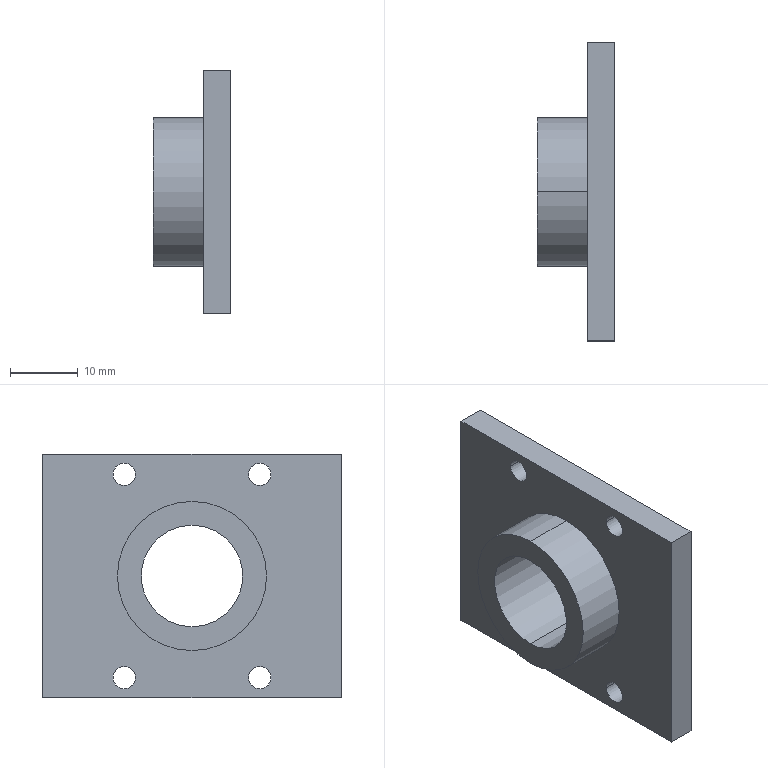Part | SolidWorks | features BaseBody 1 | 1 solid | 19 faces | box 11.5 x 44 x 36 mm | volume 7018 mm3 | cylinder 12 | plane 7 | commonest cylinder face diameters 3.3 x8 15 x2 22 x2
STEP:
#1=CARTESIAN_POINT('',(-2.,-11.65,33.));
#2=VERTEX_POINT('',#1);
#3=CARTESIAN_POINT('',(-2.,-8.35,33.));
#4=VERTEX_POINT('',#3);
#5=CARTESIAN_POINT('',(-2.,-10.,33.));
#6=DIRECTION('',(1.,0.,0.));
#7=DIRECTION('',(0.,1.,0.));
#8=AXIS2_PLACEMENT_3D('',#5,#6,#7);
#9=CIRCLE('',#8,1.65);
#10=EDGE_CURVE('',#2,#4,#9,.T.);
#11=ORIENTED_EDGE('',*,*,#10,.F.);
#12=CARTESIAN_POINT('',(2.,-11.65,33.));
#13=VERTEX_POINT('',#12);
#14=CARTESIAN_POINT('',(-14.2,-11.65,33.));
#15=DIRECTION('',(1.,0.,0.));
#16=VECTOR('',#15,1000.);
#17=LINE('',#14,#16);
#18=EDGE_CURVE('',#2,#13,#17,.T.);
#19=ORIENTED_EDGE('',*,*,#18,.T.);
#20=CARTESIAN_POINT('',(2.,-8.35,33.));
#21=VERTEX_POINT('',#20);
#22=CARTESIAN_POINT('',(2.,-10.,33.));
#23=DIRECTION('',(-1.,0.,0.));
#24=DIRECTION('',(0.,1.,0.));
#25=AXIS2_PLACEMENT_3D('',#22,#23,#24);
#26=CIRCLE('',#25,1.65);
#27=EDGE_CURVE('',#21,#13,#26,.T.);
#28=ORIENTED_EDGE('',*,*,#27,.F.);
#29=CARTESIAN_POINT('',(-14.2,-8.35,33.));
#30=DIRECTION('',(1.,0.,0.));
#31=VECTOR('',#30,1000.);
#32=LINE('',#29,#31);
#33=EDGE_CURVE('',#4,#21,#32,.T.);
#34=ORIENTED_EDGE('',*,*,#33,.F.);
#35=EDGE_LOOP('',(#11,#19,#28,#34));
#36=FACE_OUTER_BOUND('',#35,.T.);
#37=CARTESIAN_POINT('',(-14.2,-10.,33.));
#38=DIRECTION('',(1.,0.,0.));
#39=DIRECTION('',(0.,1.,0.));
#40=AXIS2_PLACEMENT_3D('',#37,#38,#39);
#41=CYLINDRICAL_SURFACE('',#40,1.65);
#42=ADVANCED_FACE('',(#36),#41,.F.);
#43=CARTESIAN_POINT('',(-9.5,0.,25.5));
#44=VERTEX_POINT('',#43);
#45=CARTESIAN_POINT('',(-9.5,0.,10.5));
#46=VERTEX_POINT('',#45);
#47=CARTESIAN_POINT('',(-9.5,0.,18.));
#48=DIRECTION('',(1.,0.,0.));
#49=DIRECTION('',(0.,0.,-1.));
#50=AXIS2_PLACEMENT_3D('',#47,#48,#49);
#51=CIRCLE('',#50,7.5);
#52=EDGE_CURVE('',#44,#46,#51,.T.);
#53=ORIENTED_EDGE('',*,*,#52,.F.);
#54=CARTESIAN_POINT('',(2.,0.,25.5));
#55=VERTEX_POINT('',#54);
#56=CARTESIAN_POINT('',(-3.,0.,25.5));
#57=DIRECTION('',(1.,0.,0.));
#58=VECTOR('',#57,1000.);
#59=LINE('',#56,#58);
#60=EDGE_CURVE('',#44,#55,#59,.T.);
#61=ORIENTED_EDGE('',*,*,#60,.T.);
#62=CARTESIAN_POINT('',(2.,0.,10.5));
#63=VERTEX_POINT('',#62);
#64=CARTESIAN_POINT('',(2.,0.,18.));
#65=DIRECTION('',(-1.,0.,0.));
#66=DIRECTION('',(0.,0.,-1.));
#67=AXIS2_PLACEMENT_3D('',#64,#65,#66);
#68=CIRCLE('',#67,7.5);
#69=EDGE_CURVE('',#63,#55,#68,.T.);
#70=ORIENTED_EDGE('',*,*,#69,.F.);
#71=CARTESIAN_POINT('',(-3.,0.,10.5));
#72=DIRECTION('',(1.,0.,0.));
#73=VECTOR('',#72,1000.);
#74=LINE('',#71,#73);
#75=EDGE_CURVE('',#46,#63,#74,.T.);
#76=ORIENTED_EDGE('',*,*,#75,.F.);
#77=EDGE_LOOP('',(#53,#61,#70,#76));
#78=FACE_OUTER_BOUND('',#77,.T.);
#79=CARTESIAN_POINT('',(-3.,0.,18.));
#80=DIRECTION('',(1.,0.,0.));
#81=DIRECTION('',(0.,0.,-1.));
#82=AXIS2_PLACEMENT_3D('',#79,#80,#81);
#83=CYLINDRICAL_SURFACE('',#82,7.5);
#84=ADVANCED_FACE('',(#78),#83,.F.);
#85=CARTESIAN_POINT('',(-2.,-11.65,3.));
#86=VERTEX_POINT('',#85);
#87=CARTESIAN_POINT('',(-2.,-8.35,3.));
#88=VERTEX_POINT('',#87);
#89=CARTESIAN_POINT('',(-2.,-10.,3.));
#90=DIRECTION('',(1.,0.,0.));
#91=DIRECTION('',(0.,1.,0.));
#92=AXIS2_PLACEMENT_3D('',#89,#90,#91);
#93=CIRCLE('',#92,1.65);
#94=EDGE_CURVE('',#86,#88,#93,.T.);
#95=ORIENTED_EDGE('',*,*,#94,.F.);
#96=CARTESIAN_POINT('',(2.,-11.65,3.));
#97=VERTEX_POINT('',#96);
#98=CARTESIAN_POINT('',(-14.2,-11.65,3.));
#99=DIRECTION('',(1.,0.,0.));
#100=VECTOR('',#99,1000.);
#101=LINE('',#98,#100);
#102=EDGE_CURVE('',#86,#97,#101,.T.);
#103=ORIENTED_EDGE('',*,*,#102,.T.);
#104=CARTESIAN_POINT('',(2.,-8.35,3.));
#105=VERTEX_POINT('',#104);
#106=CARTESIAN_POINT('',(2.,-10.,3.));
#107=DIRECTION('',(-1.,0.,0.));
#108=DIRECTION('',(0.,1.,0.));
#109=AXIS2_PLACEMENT_3D('',#106,#107,#108);
#110=CIRCLE('',#109,1.65);
#111=EDGE_CURVE('',#105,#97,#110,.T.);
#112=ORIENTED_EDGE('',*,*,#111,.F.);
#113=CARTESIAN_POINT('',(-14.2,-8.35,3.));
#114=DIRECTION('',(1.,0.,0.));
#115=VECTOR('',#114,1000.);
#116=LINE('',#113,#115);
#117=EDGE_CURVE('',#88,#105,#116,.T.);
#118=ORIENTED_EDGE('',*,*,#117,.F.);
#119=EDGE_LOOP('',(#95,#103,#112,#118));
#120=FACE_OUTER_BOUND('',#119,.T.);
#121=CARTESIAN_POINT('',(-14.2,-10.,3.));
#122=DIRECTION('',(1.,0.,0.));
#123=DIRECTION('',(0.,1.,0.));
#124=AXIS2_PLACEMENT_3D('',#121,#122,#123);
#125=CYLINDRICAL_SURFACE('',#124,1.65);
#126=ADVANCED_FACE('',(#120),#125,.F.);
#127=CARTESIAN_POINT('',(-2.,8.35,33.));
#128=VERTEX_POINT('',#127);
#129=CARTESIAN_POINT('',(-2.,11.65,33.));
#130=VERTEX_POINT('',#129);
#131=CARTESIAN_POINT('',(-2.,10.,33.));
#132=DIRECTION('',(1.,0.,0.));
#133=DIRECTION('',(0.,1.,0.));
#134=AXIS2_PLACEMENT_3D('',#131,#132,#133);
#135=CIRCLE('',#134,1.65);
#136=EDGE_CURVE('',#128,#130,#135,.T.);
#137=ORIENTED_EDGE('',*,*,#136,.F.);
#138=CARTESIAN_POINT('',(2.,8.35,33.));
#139=VERTEX_POINT('',#138);
#140=CARTESIAN_POINT('',(-14.2,8.35,33.));
#141=DIRECTION('',(1.,0.,0.));
#142=VECTOR('',#141,1000.);
#143=LINE('',#140,#142);
#144=EDGE_CURVE('',#128,#139,#143,.T.);
#145=ORIENTED_EDGE('',*,*,#144,.T.);
#146=CARTESIAN_POINT('',(2.,11.65,33.));
#147=VERTEX_POINT('',#146);
#148=CARTESIAN_POINT('',(2.,10.,33.));
#149=DIRECTION('',(-1.,0.,0.));
#150=DIRECTION('',(0.,1.,0.));
#151=AXIS2_PLACEMENT_3D('',#148,#149,#150);
#152=CIRCLE('',#151,1.65);
#153=EDGE_CURVE('',#147,#139,#152,.T.);
#154=ORIENTED_EDGE('',*,*,#153,.F.);
#155=CARTESIAN_POINT('',(-14.2,11.65,33.));
#156=DIRECTION('',(1.,0.,0.));
#157=VECTOR('',#156,1000.);
#158=LINE('',#155,#157);
#159=EDGE_CURVE('',#130,#147,#158,.T.);
#160=ORIENTED_EDGE('',*,*,#159,.F.);
#161=EDGE_LOOP('',(#137,#145,#154,#160));
#162=FACE_OUTER_BOUND('',#161,.T.);
#163=CARTESIAN_POINT('',(-14.2,10.,33.));
#164=DIRECTION('',(1.,0.,0.));
#165=DIRECTION('',(0.,1.,0.));
#166=AXIS2_PLACEMENT_3D('',#163,#164,#165);
#167=CYLINDRICAL_SURFACE('',#166,1.65);
#168=ADVANCED_FACE('',(#162),#167,.F.);
#169=CARTESIAN_POINT('',(-2.,8.35,3.));
#170=VERTEX_POINT('',#169);
#171=CARTESIAN_POINT('',(-2.,11.65,3.));
#172=VERTEX_POINT('',#171);
#173=CARTESIAN_POINT('',(-2.,10.,3.));
#174=DIRECTION('',(1.,0.,0.));
#175=DIRECTION('',(0.,1.,0.));
#176=AXIS2_PLACEMENT_3D('',#173,#174,#175);
#177=CIRCLE('',#176,1.65);
#178=EDGE_CURVE('',#170,#172,#177,.T.);
#179=ORIENTED_EDGE('',*,*,#178,.F.);
#180=CARTESIAN_POINT('',(2.,8.35,3.));
#181=VERTEX_POINT('',#180);
#182=CARTESIAN_POINT('',(-14.2,8.35,3.));
#183=DIRECTION('',(1.,0.,0.));
#184=VECTOR('',#183,1000.);
#185=LINE('',#182,#184);
#186=EDGE_CURVE('',#170,#181,#185,.T.);
#187=ORIENTED_EDGE('',*,*,#186,.T.);
#188=CARTESIAN_POINT('',(2.,11.65,3.));
#189=VERTEX_POINT('',#188);
#190=CARTESIAN_POINT('',(2.,10.,3.));
#191=DIRECTION('',(-1.,0.,0.));
#192=DIRECTION('',(0.,1.,0.));
#193=AXIS2_PLACEMENT_3D('',#190,#191,#192);
#194=CIRCLE('',#193,1.65);
#195=EDGE_CURVE('',#189,#181,#194,.T.);
#196=ORIENTED_EDGE('',*,*,#195,.F.);
#197=CARTESIAN_POINT('',(-14.2,11.65,3.));
#198=DIRECTION('',(1.,0.,0.));
#199=VECTOR('',#198,1000.);
#200=LINE('',#197,#199);
#201=EDGE_CURVE('',#172,#189,#200,.T.);
#202=ORIENTED_EDGE('',*,*,#201,.F.);
#203=EDGE_LOOP('',(#179,#187,#196,#202));
#204=FACE_OUTER_BOUND('',#203,.T.);
#205=CARTESIAN_POINT('',(-14.2,10.,3.));
#206=DIRECTION('',(1.,0.,0.));
#207=DIRECTION('',(0.,1.,0.));
#208=AXIS2_PLACEMENT_3D('',#205,#206,#207);
#209=CYLINDRICAL_SURFACE('',#208,1.65);
#210=ADVANCED_FACE('',(#204),#209,.F.);
#211=CARTESIAN_POINT('',(-9.5,0.,7.));
#212=VERTEX_POINT('',#211);
#213=CARTESIAN_POINT('',(-9.5,0.,29.));
#214=VERTEX_POINT('',#213);
#215=CARTESIAN_POINT('',(-9.5,0.,18.));
#216=DIRECTION('',(1.,0.,0.));
#217=DIRECTION('',(0.,0.,-1.));
#218=AXIS2_PLACEMENT_3D('',#215,#216,#217);
#219=CIRCLE('',#218,11.);
#220=EDGE_CURVE('',#212,#214,#219,.T.);
#221=ORIENTED_EDGE('',*,*,#220,.T.);
#222=CARTESIAN_POINT('',(-2.,0.,29.));
#223=VERTEX_POINT('',#222);
#224=CARTESIAN_POINT('',(-9.5,0.,29.));
#225=DIRECTION('',(1.,0.,0.));
#226=VECTOR('',#225,1000.);
#227=LINE('',#224,#226);
#228=EDGE_CURVE('',#214,#223,#227,.T.);
#229=ORIENTED_EDGE('',*,*,#228,.T.);
#230=CARTESIAN_POINT('',(-2.,0.,7.));
#231=VERTEX_POINT('',#230);
#232=CARTESIAN_POINT('',(-2.,0.,18.));
#233=DIRECTION('',(-1.,0.,0.));
#234=DIRECTION('',(0.,0.,-1.));
#235=AXIS2_PLACEMENT_3D('',#232,#233,#234);
#236=CIRCLE('',#235,11.);
#237=EDGE_CURVE('',#223,#231,#236,.T.);
#238=ORIENTED_EDGE('',*,*,#237,.T.);
#239=CARTESIAN_POINT('',(-9.5,0.,7.));
#240=DIRECTION('',(1.,0.,0.));
#241=VECTOR('',#240,1000.);
#242=LINE('',#239,#241);
#243=EDGE_CURVE('',#212,#231,#242,.T.);
#244=ORIENTED_EDGE('',*,*,#243,.F.);
#245=EDGE_LOOP('',(#221,#229,#238,#244));
#246=FACE_OUTER_BOUND('',#245,.T.);
#247=CARTESIAN_POINT('',(-9.5,0.,18.));
#248=DIRECTION('',(1.,0.,0.));
#249=DIRECTION('',(0.,0.,-1.));
#250=AXIS2_PLACEMENT_3D('',#247,#248,#249);
#251=CYLINDRICAL_SURFACE('',#250,11.);
#252=ADVANCED_FACE('',(#246),#251,.T.);
#253=ORIENTED_EDGE('',*,*,#27,.T.);
#254=CARTESIAN_POINT('',(2.,-10.,33.));
#255=DIRECTION('',(-1.,0.,0.));
#256=DIRECTION('',(0.,1.,0.));
#257=AXIS2_PLACEMENT_3D('',#254,#255,#256);
#258=CIRCLE('',#257,1.65);
#259=EDGE_CURVE('',#13,#21,#258,.T.);
#260=ORIENTED_EDGE('',*,*,#259,.T.);
#261=EDGE_LOOP('',(#253,#260));
#262=FACE_BOUND('',#261,.T.);
#263=ORIENTED_EDGE('',*,*,#69,.T.);
#264=CARTESIAN_POINT('',(2.,0.,18.));
#265=DIRECTION('',(-1.,0.,0.));
#266=DIRECTION('',(0.,0.,-1.));
#267=AXIS2_PLACEMENT_3D('',#264,#265,#266);
#268=CIRCLE('',#267,7.5);
#269=EDGE_CURVE('',#55,#63,#268,.T.);
#270=ORIENTED_EDGE('',*,*,#269,.T.);
#271=EDGE_LOOP('',(#263,#270));
#272=FACE_BOUND('',#271,.T.);
#273=ORIENTED_EDGE('',*,*,#111,.T.);
#274=CARTESIAN_POINT('',(2.,-10.,3.));
#275=DIRECTION('',(-1.,0.,0.));
#276=DIRECTION('',(0.,1.,0.));
#277=AXIS2_PLACEMENT_3D('',#274,#275,#276);
#278=CIRCLE('',#277,1.65);
#279=EDGE_CURVE('',#97,#105,#278,.T.);
#280=ORIENTED_EDGE('',*,*,#279,.T.);
#281=EDGE_LOOP('',(#273,#280));
#282=FACE_BOUND('',#281,.T.);
#283=ORIENTED_EDGE('',*,*,#153,.T.);
#284=CARTESIAN_POINT('',(2.,10.,33.));
#285=DIRECTION('',(-1.,0.,0.));
#286=DIRECTION('',(0.,1.,0.));
#287=AXIS2_PLACEMENT_3D('',#284,#285,#286);
#288=CIRCLE('',#287,1.65);
#289=EDGE_CURVE('',#139,#147,#288,.T.);
#290=ORIENTED_EDGE('',*,*,#289,.T.);
#291=EDGE_LOOP('',(#283,#290));
#292=FACE_BOUND('',#291,.T.);
#293=ORIENTED_EDGE('',*,*,#195,.T.);
#294=CARTESIAN_POINT('',(2.,10.,3.));
#295=DIRECTION('',(-1.,0.,0.));
#296=DIRECTION('',(0.,1.,0.));
#297=AXIS2_PLACEMENT_3D('',#294,#295,#296);
#298=CIRCLE('',#297,1.65);
#299=EDGE_CURVE('',#181,#189,#298,.T.);
#300=ORIENTED_EDGE('',*,*,#299,.T.);
#301=EDGE_LOOP('',(#293,#300));
#302=FACE_BOUND('',#301,.T.);
#303=CARTESIAN_POINT('',(2.,22.,0.));
#304=VERTEX_POINT('',#303);
#305=CARTESIAN_POINT('',(2.,22.,36.));
#306=VERTEX_POINT('',#305);
#307=CARTESIAN_POINT('',(2.,22.,0.));
#308=DIRECTION('',(0.,0.,1.));
#309=VECTOR('',#308,1000.);
#310=LINE('',#307,#309);
#311=EDGE_CURVE('',#304,#306,#310,.T.);
#312=ORIENTED_EDGE('',*,*,#311,.T.);
#313=CARTESIAN_POINT('',(2.,-22.,36.));
#314=VERTEX_POINT('',#313);
#315=CARTESIAN_POINT('',(2.,-22.,36.));
#316=DIRECTION('',(0.,-1.,0.));
#317=VECTOR('',#316,1000.);
#318=LINE('',#315,#317);
#319=EDGE_CURVE('',#306,#314,#318,.T.);
#320=ORIENTED_EDGE('',*,*,#319,.T.);
#321=CARTESIAN_POINT('',(2.,-22.,0.));
#322=VERTEX_POINT('',#321);
#323=CARTESIAN_POINT('',(2.,-22.,0.));
#324=DIRECTION('',(0.,0.,-1.));
#325=VECTOR('',#324,1000.);
#326=LINE('',#323,#325);
#327=EDGE_CURVE('',#314,#322,#326,.T.);
#328=ORIENTED_EDGE('',*,*,#327,.T.);
#329=CARTESIAN_POINT('',(2.,-22.,0.));
#330=DIRECTION('',(0.,1.,0.));
#331=VECTOR('',#330,1000.);
#332=LINE('',#329,#331);
#333=EDGE_CURVE('',#322,#304,#332,.T.);
#334=ORIENTED_EDGE('',*,*,#333,.T.);
#335=EDGE_LOOP('',(#312,#320,#328,#334));
#336=FACE_OUTER_BOUND('',#335,.T.);
#337=CARTESIAN_POINT('',(2.,-22.,0.));
#338=DIRECTION('',(1.,0.,0.));
#339=DIRECTION('',(0.,0.,-1.));
#340=AXIS2_PLACEMENT_3D('',#337,#338,#339);
#341=PLANE('',#340);
#342=ADVANCED_FACE('',(#262,#272,#282,#292,#302,#336),#341,.T.);
#343=ORIENTED_EDGE('',*,*,#18,.F.);
#344=CARTESIAN_POINT('',(-2.,-10.,33.));
#345=DIRECTION('',(1.,0.,0.));
#346=DIRECTION('',(0.,1.,0.));
#347=AXIS2_PLACEMENT_3D('',#344,#345,#346);
#348=CIRCLE('',#347,1.65);
#349=EDGE_CURVE('',#4,#2,#348,.T.);
#350=ORIENTED_EDGE('',*,*,#349,.F.);
#351=ORIENTED_EDGE('',*,*,#33,.T.);
#352=ORIENTED_EDGE('',*,*,#259,.F.);
#353=EDGE_LOOP('',(#343,#350,#351,#352));
#354=FACE_OUTER_BOUND('',#353,.T.);
#355=CARTESIAN_POINT('',(-14.2,-10.,33.));
#356=DIRECTION('',(1.,0.,0.));
#357=DIRECTION('',(0.,1.,0.));
#358=AXIS2_PLACEMENT_3D('',#355,#356,#357);
#359=CYLINDRICAL_SURFACE('',#358,1.65);
#360=ADVANCED_FACE('',(#354),#359,.F.);
#361=ORIENTED_EDGE('',*,*,#60,.F.);
#362=CARTESIAN_POINT('',(-9.5,0.,18.));
#363=DIRECTION('',(1.,0.,0.));
#364=DIRECTION('',(0.,0.,-1.));
#365=AXIS2_PLACEMENT_3D('',#362,#363,#364);
#366=CIRCLE('',#365,7.5);
#367=EDGE_CURVE('',#46,#44,#366,.T.);
#368=ORIENTED_EDGE('',*,*,#367,.F.);
#369=ORIENTED_EDGE('',*,*,#75,.T.);
#370=ORIENTED_EDGE('',*,*,#269,.F.);
#371=EDGE_LOOP('',(#361,#368,#369,#370));
#372=FACE_OUTER_BOUND('',#371,.T.);
#373=CARTESIAN_POINT('',(-3.,0.,18.));
#374=DIRECTION('',(1.,0.,0.));
#375=DIRECTION('',(0.,0.,-1.));
#376=AXIS2_PLACEMENT_3D('',#373,#374,#375);
#377=CYLINDRICAL_SURFACE('',#376,7.5);
#378=ADVANCED_FACE('',(#372),#377,.F.);
#379=ORIENTED_EDGE('',*,*,#102,.F.);
#380=CARTESIAN_POINT('',(-2.,-10.,3.));
#381=DIRECTION('',(1.,0.,0.));
#382=DIRECTION('',(0.,1.,0.));
#383=AXIS2_PLACEMENT_3D('',#380,#381,#382);
#384=CIRCLE('',#383,1.65);
#385=EDGE_CURVE('',#88,#86,#384,.T.);
#386=ORIENTED_EDGE('',*,*,#385,.F.);
#387=ORIENTED_EDGE('',*,*,#117,.T.);
#388=ORIENTED_EDGE('',*,*,#279,.F.);
#389=EDGE_LOOP('',(#379,#386,#387,#388));
#390=FACE_OUTER_BOUND('',#389,.T.);
#391=CARTESIAN_POINT('',(-14.2,-10.,3.));
#392=DIRECTION('',(1.,0.,0.));
#393=DIRECTION('',(0.,1.,0.));
#394=AXIS2_PLACEMENT_3D('',#391,#392,#393);
#395=CYLINDRICAL_SURFACE('',#394,1.65);
#396=ADVANCED_FACE('',(#390),#395,.F.);
#397=ORIENTED_EDGE('',*,*,#144,.F.);
#398=CARTESIAN_POINT('',(-2.,10.,33.));
#399=DIRECTION('',(1.,0.,0.));
#400=DIRECTION('',(0.,1.,0.));
#401=AXIS2_PLACEMENT_3D('',#398,#399,#400);
#402=CIRCLE('',#401,1.65);
#403=EDGE_CURVE('',#130,#128,#402,.T.);
#404=ORIENTED_EDGE('',*,*,#403,.F.);
#405=ORIENTED_EDGE('',*,*,#159,.T.);
#406=ORIENTED_EDGE('',*,*,#289,.F.);
#407=EDGE_LOOP('',(#397,#404,#405,#406));
#408=FACE_OUTER_BOUND('',#407,.T.);
#409=CARTESIAN_POINT('',(-14.2,10.,33.));
#410=DIRECTION('',(1.,0.,0.));
#411=DIRECTION('',(0.,1.,0.));
#412=AXIS2_PLACEMENT_3D('',#409,#410,#411);
#413=CYLINDRICAL_SURFACE('',#412,1.65);
#414=ADVANCED_FACE('',(#408),#413,.F.);
#415=ORIENTED_EDGE('',*,*,#186,.F.);
#416=CARTESIAN_POINT('',(-2.,10.,3.));
#417=DIRECTION('',(1.,0.,0.));
#418=DIRECTION('',(0.,1.,0.));
#419=AXIS2_PLACEMENT_3D('',#416,#417,#418);
#420=CIRCLE('',#419,1.65);
#421=EDGE_CURVE('',#172,#170,#420,.T.);
#422=ORIENTED_EDGE('',*,*,#421,.F.);
#423=ORIENTED_EDGE('',*,*,#201,.T.);
#424=ORIENTED_EDGE('',*,*,#299,.F.);
#425=EDGE_LOOP('',(#415,#422,#423,#424));
#426=FACE_OUTER_BOUND('',#425,.T.);
#427=CARTESIAN_POINT('',(-14.2,10.,3.));
#428=DIRECTION('',(1.,0.,0.));
#429=DIRECTION('',(0.,1.,0.));
#430=AXIS2_PLACEMENT_3D('',#427,#428,#429);
#431=CYLINDRICAL_SURFACE('',#430,1.65);
#432=ADVANCED_FACE('',(#426),#431,.F.);
#433=ORIENTED_EDGE('',*,*,#319,.F.);
#434=CARTESIAN_POINT('',(-2.,22.,36.));
#435=VERTEX_POINT('',#434);
#436=CARTESIAN_POINT('',(-2.,22.,36.));
#437=DIRECTION('',(-1.,0.,0.));
#438=VECTOR('',#437,1000.);
#439=LINE('',#436,#438);
#440=EDGE_CURVE('',#306,#435,#439,.T.);
#441=ORIENTED_EDGE('',*,*,#440,.T.);
#442=CARTESIAN_POINT('',(-2.,-22.,36.));
#443=VERTEX_POINT('',#442);
#444=CARTESIAN_POINT('',(-2.,-22.,36.));
#445=DIRECTION('',(0.,-1.,0.));
#446=VECTOR('',#445,1000.);
#447=LINE('',#444,#446);
#448=EDGE_CURVE('',#435,#443,#447,.T.);
#449=ORIENTED_EDGE('',*,*,#448,.T.);
#450=CARTESIAN_POINT('',(-2.,-22.,36.));
#451=DIRECTION('',(1.,0.,0.));
#452=VECTOR('',#451,1000.);
#453=LINE('',#450,#452);
#454=EDGE_CURVE('',#443,#314,#453,.T.);
#455=ORIENTED_EDGE('',*,*,#454,.T.);
#456=EDGE_LOOP('',(#433,#441,#449,#455));
#457=FACE_OUTER_BOUND('',#456,.T.);
#458=CARTESIAN_POINT('',(-2.,-22.,36.));
#459=DIRECTION('',(0.,0.,1.));
#460=DIRECTION('',(1.,0.,0.));
#461=AXIS2_PLACEMENT_3D('',#458,#459,#460);
#462=PLANE('',#461);
#463=ADVANCED_FACE('',(#457),#462,.T.);
#464=ORIENTED_EDGE('',*,*,#440,.F.);
#465=ORIENTED_EDGE('',*,*,#311,.F.);
#466=CARTESIAN_POINT('',(-2.,22.,0.));
#467=VERTEX_POINT('',#466);
#468=CARTESIAN_POINT('',(-2.,22.,0.));
#469=DIRECTION('',(-1.,0.,0.));
#470=VECTOR('',#469,1000.);
#471=LINE('',#468,#470);
#472=EDGE_CURVE('',#304,#467,#471,.T.);
#473=ORIENTED_EDGE('',*,*,#472,.T.);
#474=CARTESIAN_POINT('',(-2.,22.,0.));
#475=DIRECTION('',(0.,0.,1.));
#476=VECTOR('',#475,1000.);
#477=LINE('',#474,#476);
#478=EDGE_CURVE('',#467,#435,#477,.T.);
#479=ORIENTED_EDGE('',*,*,#478,.T.);
#480=EDGE_LOOP('',(#464,#465,#473,#479));
#481=FACE_OUTER_BOUND('',#480,.T.);
#482=CARTESIAN_POINT('',(-2.,22.,0.));
#483=DIRECTION('',(0.,1.,0.));
#484=DIRECTION('',(0.,0.,1.));
#485=AXIS2_PLACEMENT_3D('',#482,#483,#484);
#486=PLANE('',#485);
#487=ADVANCED_FACE('',(#481),#486,.T.);
#488=ORIENTED_EDGE('',*,*,#333,.F.);
#489=CARTESIAN_POINT('',(-2.,-22.,0.));
#490=VERTEX_POINT('',#489);
#491=CARTESIAN_POINT('',(-2.,-22.,0.));
#492=DIRECTION('',(1.,0.,0.));
#493=VECTOR('',#492,1000.);
#494=LINE('',#491,#493);
#495=EDGE_CURVE('',#490,#322,#494,.T.);
#496=ORIENTED_EDGE('',*,*,#495,.F.);
#497=CARTESIAN_POINT('',(-2.,-22.,0.));
#498=DIRECTION('',(0.,-1.,0.));
#499=VECTOR('',#498,1000.);
#500=LINE('',#497,#499);
#501=EDGE_CURVE('',#467,#490,#500,.T.);
#502=ORIENTED_EDGE('',*,*,#501,.F.);
#503=ORIENTED_EDGE('',*,*,#472,.F.);
#504=EDGE_LOOP('',(#488,#496,#502,#503));
#505=FACE_OUTER_BOUND('',#504,.T.);
#506=CARTESIAN_POINT('',(-2.,-22.,0.));
#507=DIRECTION('',(0.,0.,1.));
#508=DIRECTION('',(1.,0.,0.));
#509=AXIS2_PLACEMENT_3D('',#506,#507,#508);
#510=PLANE('',#509);
#511=ADVANCED_FACE('',(#505),#510,.F.);
#512=ORIENTED_EDGE('',*,*,#454,.F.);
#513=CARTESIAN_POINT('',(-2.,-22.,0.));
#514=DIRECTION('',(0.,0.,1.));
#515=VECTOR('',#514,1000.);
#516=LINE('',#513,#515);
#517=EDGE_CURVE('',#490,#443,#516,.T.);
#518=ORIENTED_EDGE('',*,*,#517,.F.);
#519=ORIENTED_EDGE('',*,*,#495,.T.);
#520=ORIENTED_EDGE('',*,*,#327,.F.);
#521=EDGE_LOOP('',(#512,#518,#519,#520));
#522=FACE_OUTER_BOUND('',#521,.T.);
#523=CARTESIAN_POINT('',(-2.,-22.,0.));
#524=DIRECTION('',(0.,1.,0.));
#525=DIRECTION('',(0.,0.,1.));
#526=AXIS2_PLACEMENT_3D('',#523,#524,#525);
#527=PLANE('',#526);
#528=ADVANCED_FACE('',(#522),#527,.F.);
#529=ORIENTED_EDGE('',*,*,#349,.T.);
#530=ORIENTED_EDGE('',*,*,#10,.T.);
#531=EDGE_LOOP('',(#529,#530));
#532=FACE_BOUND('',#531,.T.);
#533=CARTESIAN_POINT('',(-2.,0.,18.));
#534=DIRECTION('',(-1.,0.,0.));
#535=DIRECTION('',(0.,0.,-1.));
#536=AXIS2_PLACEMENT_3D('',#533,#534,#535);
#537=CIRCLE('',#536,11.);
#538=EDGE_CURVE('',#231,#223,#537,.T.);
#539=ORIENTED_EDGE('',*,*,#538,.F.);
#540=ORIENTED_EDGE('',*,*,#237,.F.);
#541=EDGE_LOOP('',(#539,#540));
#542=FACE_BOUND('',#541,.T.);
#543=ORIENTED_EDGE('',*,*,#385,.T.);
#544=ORIENTED_EDGE('',*,*,#94,.T.);
#545=EDGE_LOOP('',(#543,#544));
#546=FACE_BOUND('',#545,.T.);
#547=ORIENTED_EDGE('',*,*,#403,.T.);
#548=ORIENTED_EDGE('',*,*,#136,.T.);
#549=EDGE_LOOP('',(#547,#548));
#550=FACE_BOUND('',#549,.T.);
#551=ORIENTED_EDGE('',*,*,#421,.T.);
#552=ORIENTED_EDGE('',*,*,#178,.T.);
#553=EDGE_LOOP('',(#551,#552));
#554=FACE_BOUND('',#553,.T.);
#555=ORIENTED_EDGE('',*,*,#478,.F.);
#556=ORIENTED_EDGE('',*,*,#501,.T.);
#557=ORIENTED_EDGE('',*,*,#517,.T.);
#558=ORIENTED_EDGE('',*,*,#448,.F.);
#559=EDGE_LOOP('',(#555,#556,#557,#558));
#560=FACE_OUTER_BOUND('',#559,.T.);
#561=CARTESIAN_POINT('',(-2.,-22.,0.));
#562=DIRECTION('',(1.,0.,0.));
#563=DIRECTION('',(0.,0.,-1.));
#564=AXIS2_PLACEMENT_3D('',#561,#562,#563);
#565=PLANE('',#564);
#566=ADVANCED_FACE('',(#532,#542,#546,#550,#554,#560),#565,.F.);
#567=ORIENTED_EDGE('',*,*,#367,.T.);
#568=ORIENTED_EDGE('',*,*,#52,.T.);
#569=EDGE_LOOP('',(#567,#568));
#570=FACE_BOUND('',#569,.T.);
#571=ORIENTED_EDGE('',*,*,#220,.F.);
#572=CARTESIAN_POINT('',(-9.5,0.,18.));
#573=DIRECTION('',(1.,0.,0.));
#574=DIRECTION('',(0.,0.,-1.));
#575=AXIS2_PLACEMENT_3D('',#572,#573,#574);
#576=CIRCLE('',#575,11.);
#577=EDGE_CURVE('',#214,#212,#576,.T.);
#578=ORIENTED_EDGE('',*,*,#577,.F.);
#579=EDGE_LOOP('',(#571,#578));
#580=FACE_OUTER_BOUND('',#579,.T.);
#581=CARTESIAN_POINT('',(-9.5,0.,18.));
#582=DIRECTION('',(1.,0.,0.));
#583=DIRECTION('',(0.,0.,-1.));
#584=AXIS2_PLACEMENT_3D('',#581,#582,#583);
#585=PLANE('',#584);
#586=ADVANCED_FACE('',(#570,#580),#585,.F.);
#587=ORIENTED_EDGE('',*,*,#228,.F.);
#588=ORIENTED_EDGE('',*,*,#577,.T.);
#589=ORIENTED_EDGE('',*,*,#243,.T.);
#590=ORIENTED_EDGE('',*,*,#538,.T.);
#591=EDGE_LOOP('',(#587,#588,#589,#590));
#592=FACE_OUTER_BOUND('',#591,.T.);
#593=CARTESIAN_POINT('',(-9.5,0.,18.));
#594=DIRECTION('',(1.,0.,0.));
#595=DIRECTION('',(0.,0.,-1.));
#596=AXIS2_PLACEMENT_3D('',#593,#594,#595);
#597=CYLINDRICAL_SURFACE('',#596,11.);
#598=ADVANCED_FACE('',(#592),#597,.T.);
#599=CLOSED_SHELL('',(#42,#84,#126,#168,#210,#252,#342,#360,#378,#396,#414,#432,#463,#487,#511,#528,#566,#586,#598));
#600=MANIFOLD_SOLID_BREP('',#599);
#601=CARTESIAN_POINT('',(0.,0.,0.));
#602=DIRECTION('',(0.,0.,1.));
#603=DIRECTION('',(1.,0.,0.));
#604=AXIS2_PLACEMENT_3D('',#601,#602,#603);
#605=(LENGTH_UNIT()NAMED_UNIT(*)SI_UNIT(.MILLI.,.METRE.));
#606=UNCERTAINTY_MEASURE_WITH_UNIT(LENGTH_MEASURE(0.00001),#605,'','');
#607=(NAMED_UNIT(*)PLANE_ANGLE_UNIT()SI_UNIT($,.RADIAN.));
#608=(NAMED_UNIT(*)SI_UNIT($,.STERADIAN.)SOLID_ANGLE_UNIT());
#609=(GEOMETRIC_REPRESENTATION_CONTEXT(3)GLOBAL_UNCERTAINTY_ASSIGNED_CONTEXT((#606))GLOBAL_UNIT_ASSIGNED_CONTEXT((#605,#607,#608))REPRESENTATION_CONTEXT('',''));
#610=ADVANCED_BREP_SHAPE_REPRESENTATION('',(#600,#604),#609);